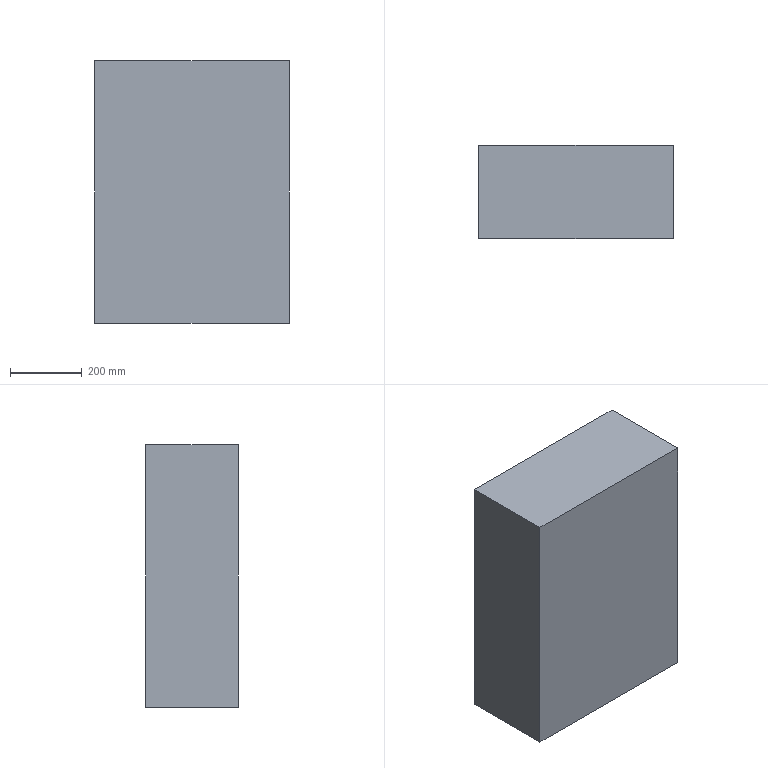Part | SolidWorks | 1 solid | 6 faces | box 545 x 260 x 735 mm | volume 104149500 mm3 | plane 6
STEP:
#1=CARTESIAN_POINT('',(-272.5,130.,367.5));
#2=VERTEX_POINT('',#1);
#3=CARTESIAN_POINT('',(-272.5,-130.,367.5));
#4=VERTEX_POINT('',#3);
#5=CARTESIAN_POINT('',(-272.5,-130.,367.5));
#6=DIRECTION('',(0.,-1.,0.));
#7=VECTOR('',#6,1000.);
#8=LINE('',#5,#7);
#9=EDGE_CURVE('',#2,#4,#8,.T.);
#10=ORIENTED_EDGE('',*,*,#9,.T.);
#11=CARTESIAN_POINT('',(272.5,-130.,367.5));
#12=VERTEX_POINT('',#11);
#13=CARTESIAN_POINT('',(272.5,-130.,367.5));
#14=DIRECTION('',(-1.,0.,0.));
#15=VECTOR('',#14,1000.);
#16=LINE('',#13,#15);
#17=EDGE_CURVE('',#12,#4,#16,.T.);
#18=ORIENTED_EDGE('',*,*,#17,.F.);
#19=CARTESIAN_POINT('',(272.5,130.,367.5));
#20=VERTEX_POINT('',#19);
#21=CARTESIAN_POINT('',(272.5,-130.,367.5));
#22=DIRECTION('',(0.,-1.,0.));
#23=VECTOR('',#22,1000.);
#24=LINE('',#21,#23);
#25=EDGE_CURVE('',#20,#12,#24,.T.);
#26=ORIENTED_EDGE('',*,*,#25,.F.);
#27=CARTESIAN_POINT('',(272.5,130.,367.5));
#28=DIRECTION('',(-1.,0.,0.));
#29=VECTOR('',#28,1000.);
#30=LINE('',#27,#29);
#31=EDGE_CURVE('',#20,#2,#30,.T.);
#32=ORIENTED_EDGE('',*,*,#31,.T.);
#33=EDGE_LOOP('',(#10,#18,#26,#32));
#34=FACE_OUTER_BOUND('',#33,.T.);
#35=CARTESIAN_POINT('',(272.5,-130.,367.5));
#36=DIRECTION('',(0.,0.,-1.));
#37=DIRECTION('',(-1.,0.,0.));
#38=AXIS2_PLACEMENT_3D('',#35,#36,#37);
#39=PLANE('',#38);
#40=ADVANCED_FACE('',(#34),#39,.F.);
#41=CARTESIAN_POINT('',(-272.5,-130.,-367.5));
#42=VERTEX_POINT('',#41);
#43=CARTESIAN_POINT('',(-272.5,-130.,-367.5));
#44=DIRECTION('',(0.,0.,-1.));
#45=VECTOR('',#44,1000.);
#46=LINE('',#43,#45);
#47=EDGE_CURVE('',#4,#42,#46,.T.);
#48=ORIENTED_EDGE('',*,*,#47,.T.);
#49=CARTESIAN_POINT('',(272.5,-130.,-367.5));
#50=VERTEX_POINT('',#49);
#51=CARTESIAN_POINT('',(272.5,-130.,-367.5));
#52=DIRECTION('',(-1.,0.,0.));
#53=VECTOR('',#52,1000.);
#54=LINE('',#51,#53);
#55=EDGE_CURVE('',#50,#42,#54,.T.);
#56=ORIENTED_EDGE('',*,*,#55,.F.);
#57=CARTESIAN_POINT('',(272.5,-130.,-367.5));
#58=DIRECTION('',(0.,0.,-1.));
#59=VECTOR('',#58,1000.);
#60=LINE('',#57,#59);
#61=EDGE_CURVE('',#12,#50,#60,.T.);
#62=ORIENTED_EDGE('',*,*,#61,.F.);
#63=ORIENTED_EDGE('',*,*,#17,.T.);
#64=EDGE_LOOP('',(#48,#56,#62,#63));
#65=FACE_OUTER_BOUND('',#64,.T.);
#66=CARTESIAN_POINT('',(272.5,-130.,-367.5));
#67=DIRECTION('',(0.,1.,0.));
#68=DIRECTION('',(0.,0.,1.));
#69=AXIS2_PLACEMENT_3D('',#66,#67,#68);
#70=PLANE('',#69);
#71=ADVANCED_FACE('',(#65),#70,.F.);
#72=CARTESIAN_POINT('',(-272.5,130.,-367.5));
#73=VERTEX_POINT('',#72);
#74=CARTESIAN_POINT('',(-272.5,-130.,-367.5));
#75=DIRECTION('',(0.,1.,0.));
#76=VECTOR('',#75,1000.);
#77=LINE('',#74,#76);
#78=EDGE_CURVE('',#42,#73,#77,.T.);
#79=ORIENTED_EDGE('',*,*,#78,.T.);
#80=CARTESIAN_POINT('',(272.5,130.,-367.5));
#81=VERTEX_POINT('',#80);
#82=CARTESIAN_POINT('',(272.5,130.,-367.5));
#83=DIRECTION('',(-1.,0.,0.));
#84=VECTOR('',#83,1000.);
#85=LINE('',#82,#84);
#86=EDGE_CURVE('',#81,#73,#85,.T.);
#87=ORIENTED_EDGE('',*,*,#86,.F.);
#88=CARTESIAN_POINT('',(272.5,-130.,-367.5));
#89=DIRECTION('',(0.,1.,0.));
#90=VECTOR('',#89,1000.);
#91=LINE('',#88,#90);
#92=EDGE_CURVE('',#50,#81,#91,.T.);
#93=ORIENTED_EDGE('',*,*,#92,.F.);
#94=ORIENTED_EDGE('',*,*,#55,.T.);
#95=EDGE_LOOP('',(#79,#87,#93,#94));
#96=FACE_OUTER_BOUND('',#95,.T.);
#97=CARTESIAN_POINT('',(272.5,-130.,-367.5));
#98=DIRECTION('',(0.,0.,1.));
#99=DIRECTION('',(1.,0.,0.));
#100=AXIS2_PLACEMENT_3D('',#97,#98,#99);
#101=PLANE('',#100);
#102=ADVANCED_FACE('',(#96),#101,.F.);
#103=CARTESIAN_POINT('',(-272.5,130.,-367.5));
#104=DIRECTION('',(0.,0.,1.));
#105=VECTOR('',#104,1000.);
#106=LINE('',#103,#105);
#107=EDGE_CURVE('',#73,#2,#106,.T.);
#108=ORIENTED_EDGE('',*,*,#107,.T.);
#109=ORIENTED_EDGE('',*,*,#31,.F.);
#110=CARTESIAN_POINT('',(272.5,130.,-367.5));
#111=DIRECTION('',(0.,0.,1.));
#112=VECTOR('',#111,1000.);
#113=LINE('',#110,#112);
#114=EDGE_CURVE('',#81,#20,#113,.T.);
#115=ORIENTED_EDGE('',*,*,#114,.F.);
#116=ORIENTED_EDGE('',*,*,#86,.T.);
#117=EDGE_LOOP('',(#108,#109,#115,#116));
#118=FACE_OUTER_BOUND('',#117,.T.);
#119=CARTESIAN_POINT('',(272.5,130.,-367.5));
#120=DIRECTION('',(0.,-1.,0.));
#121=DIRECTION('',(0.,0.,-1.));
#122=AXIS2_PLACEMENT_3D('',#119,#120,#121);
#123=PLANE('',#122);
#124=ADVANCED_FACE('',(#118),#123,.F.);
#125=ORIENTED_EDGE('',*,*,#25,.T.);
#126=ORIENTED_EDGE('',*,*,#61,.T.);
#127=ORIENTED_EDGE('',*,*,#92,.T.);
#128=ORIENTED_EDGE('',*,*,#114,.T.);
#129=EDGE_LOOP('',(#125,#126,#127,#128));
#130=FACE_OUTER_BOUND('',#129,.T.);
#131=CARTESIAN_POINT('',(272.5,0.,0.));
#132=DIRECTION('',(1.,0.,0.));
#133=DIRECTION('',(0.,0.,-1.));
#134=AXIS2_PLACEMENT_3D('',#131,#132,#133);
#135=PLANE('',#134);
#136=ADVANCED_FACE('',(#130),#135,.T.);
#137=ORIENTED_EDGE('',*,*,#9,.F.);
#138=ORIENTED_EDGE('',*,*,#107,.F.);
#139=ORIENTED_EDGE('',*,*,#78,.F.);
#140=ORIENTED_EDGE('',*,*,#47,.F.);
#141=EDGE_LOOP('',(#137,#138,#139,#140));
#142=FACE_OUTER_BOUND('',#141,.T.);
#143=CARTESIAN_POINT('',(-272.5,0.,0.));
#144=DIRECTION('',(1.,0.,0.));
#145=DIRECTION('',(0.,0.,-1.));
#146=AXIS2_PLACEMENT_3D('',#143,#144,#145);
#147=PLANE('',#146);
#148=ADVANCED_FACE('',(#142),#147,.F.);
#149=CLOSED_SHELL('',(#40,#71,#102,#124,#136,#148));
#150=MANIFOLD_SOLID_BREP('',#149);
#151=CARTESIAN_POINT('',(0.,0.,0.));
#152=DIRECTION('',(0.,0.,1.));
#153=DIRECTION('',(1.,0.,0.));
#154=AXIS2_PLACEMENT_3D('',#151,#152,#153);
#155=(LENGTH_UNIT()NAMED_UNIT(*)SI_UNIT(.MILLI.,.METRE.));
#156=UNCERTAINTY_MEASURE_WITH_UNIT(LENGTH_MEASURE(0.00001),#155,'','');
#157=(NAMED_UNIT(*)PLANE_ANGLE_UNIT()SI_UNIT($,.RADIAN.));
#158=(NAMED_UNIT(*)SI_UNIT($,.STERADIAN.)SOLID_ANGLE_UNIT());
#159=(GEOMETRIC_REPRESENTATION_CONTEXT(3)GLOBAL_UNCERTAINTY_ASSIGNED_CONTEXT((#156))GLOBAL_UNIT_ASSIGNED_CONTEXT((#155,#157,#158))REPRESENTATION_CONTEXT('',''));
#160=ADVANCED_BREP_SHAPE_REPRESENTATION('',(#150,#154),#159);